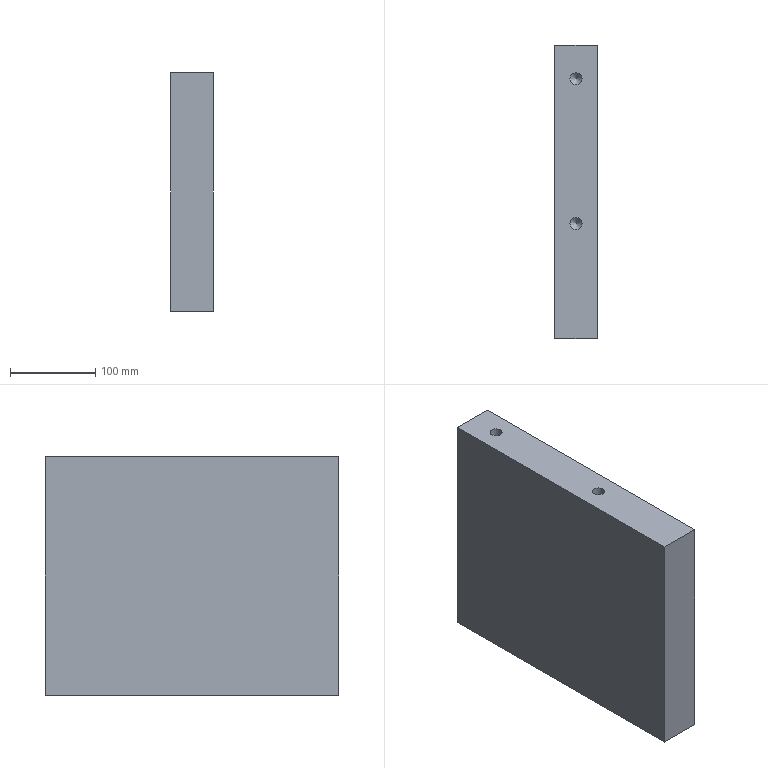Part | NX | features 29 2 | 1 solid | 14 faces | box 50 x 344.338 x 280.5 mm | volume 4804797 mm3 | plane 6 | cylinder 4 | cone 4 | commonest cylinder face diameters 14.1 x4
STEP:
#1=CARTESIAN_POINT('',(259.55,-367.5,-493.5));
#2=VERTEX_POINT('',#1);
#3=CARTESIAN_POINT('',(252.5,-367.5,-493.5));
#4=DIRECTION('',(0.,0.,1.));
#5=DIRECTION('',(1.,0.,0.));
#6=AXIS2_PLACEMENT_3D('',#3,#4,#5);
#7=CIRCLE('',#6,7.05);
#8=EDGE_CURVE('',#2,#2,#7,.T.);
#9=ORIENTED_EDGE('',*,*,#8,.T.);
#10=EDGE_LOOP('',(#9));
#11=FACE_BOUND('',#10,.T.);
#12=CARTESIAN_POINT('',(227.5,-328.162,-493.5));
#13=VERTEX_POINT('',#12);
#14=CARTESIAN_POINT('',(227.5,-672.5,-493.5));
#15=VERTEX_POINT('',#14);
#16=CARTESIAN_POINT('',(227.5,193.,-493.5));
#17=DIRECTION('',(0.,-1.,0.));
#18=VECTOR('',#17,1000.);
#19=LINE('',#16,#18);
#20=EDGE_CURVE('',#13,#15,#19,.T.);
#21=ORIENTED_EDGE('',*,*,#20,.F.);
#22=CARTESIAN_POINT('',(277.5,-328.162,-493.5));
#23=VERTEX_POINT('',#22);
#24=CARTESIAN_POINT('',(1945.,-328.162,-493.5));
#25=DIRECTION('',(1.,0.,0.));
#26=VECTOR('',#25,1000.);
#27=LINE('',#24,#26);
#28=EDGE_CURVE('',#13,#23,#27,.T.);
#29=ORIENTED_EDGE('',*,*,#28,.T.);
#30=CARTESIAN_POINT('',(277.5,-672.5,-493.5));
#31=VERTEX_POINT('',#30);
#32=CARTESIAN_POINT('',(277.5,193.,-493.5));
#33=DIRECTION('',(0.,1.,0.));
#34=VECTOR('',#33,1000.);
#35=LINE('',#32,#34);
#36=EDGE_CURVE('',#31,#23,#35,.T.);
#37=ORIENTED_EDGE('',*,*,#36,.F.);
#38=CARTESIAN_POINT('',(172.5,-672.5,-493.5));
#39=DIRECTION('',(-1.,0.,0.));
#40=VECTOR('',#39,1000.);
#41=LINE('',#38,#40);
#42=EDGE_CURVE('',#31,#15,#41,.T.);
#43=ORIENTED_EDGE('',*,*,#42,.T.);
#44=EDGE_LOOP('',(#21,#29,#37,#43));
#45=FACE_BOUND('',#44,.T.);
#46=CARTESIAN_POINT('',(259.55,-617.5,-493.5));
#47=VERTEX_POINT('',#46);
#48=CARTESIAN_POINT('',(252.5,-617.5,-493.5));
#49=DIRECTION('',(0.,0.,1.));
#50=DIRECTION('',(1.,0.,0.));
#51=AXIS2_PLACEMENT_3D('',#48,#49,#50);
#52=CIRCLE('',#51,7.05);
#53=EDGE_CURVE('',#47,#47,#52,.T.);
#54=ORIENTED_EDGE('',*,*,#53,.T.);
#55=EDGE_LOOP('',(#54));
#56=FACE_BOUND('',#55,.T.);
#57=CARTESIAN_POINT('',(1945.,0.,-493.5));
#58=DIRECTION('',(0.,0.,-1.));
#59=DIRECTION('',(1.,0.,0.));
#60=AXIS2_PLACEMENT_3D('',#57,#58,#59);
#61=PLANE('',#60);
#62=ADVANCED_FACE('',(#11,#45,#56),#61,.T.);
#63=CARTESIAN_POINT('',(259.55,-537.5,-213.));
#64=VERTEX_POINT('',#63);
#65=CARTESIAN_POINT('',(252.5,-537.5,-213.));
#66=DIRECTION('',(0.,0.,-1.));
#67=DIRECTION('',(1.,0.,0.));
#68=AXIS2_PLACEMENT_3D('',#65,#66,#67);
#69=CIRCLE('',#68,7.05);
#70=EDGE_CURVE('',#64,#64,#69,.T.);
#71=ORIENTED_EDGE('',*,*,#70,.T.);
#72=EDGE_LOOP('',(#71));
#73=FACE_BOUND('',#72,.T.);
#74=CARTESIAN_POINT('',(277.5,-328.162,-213.));
#75=VERTEX_POINT('',#74);
#76=CARTESIAN_POINT('',(277.5,-672.5,-213.));
#77=VERTEX_POINT('',#76);
#78=CARTESIAN_POINT('',(277.5,193.,-213.));
#79=DIRECTION('',(0.,-1.,0.));
#80=VECTOR('',#79,1000.);
#81=LINE('',#78,#80);
#82=EDGE_CURVE('',#75,#77,#81,.T.);
#83=ORIENTED_EDGE('',*,*,#82,.F.);
#84=CARTESIAN_POINT('',(227.5,-328.162,-213.));
#85=VERTEX_POINT('',#84);
#86=CARTESIAN_POINT('',(1945.,-328.162,-213.));
#87=DIRECTION('',(-1.,0.,0.));
#88=VECTOR('',#87,1000.);
#89=LINE('',#86,#88);
#90=EDGE_CURVE('',#75,#85,#89,.T.);
#91=ORIENTED_EDGE('',*,*,#90,.T.);
#92=CARTESIAN_POINT('',(227.5,-672.5,-213.));
#93=VERTEX_POINT('',#92);
#94=CARTESIAN_POINT('',(227.5,193.,-213.));
#95=DIRECTION('',(0.,1.,0.));
#96=VECTOR('',#95,1000.);
#97=LINE('',#94,#96);
#98=EDGE_CURVE('',#93,#85,#97,.T.);
#99=ORIENTED_EDGE('',*,*,#98,.F.);
#100=CARTESIAN_POINT('',(172.5,-672.5,-213.));
#101=DIRECTION('',(1.,0.,0.));
#102=VECTOR('',#101,1000.);
#103=LINE('',#100,#102);
#104=EDGE_CURVE('',#93,#77,#103,.T.);
#105=ORIENTED_EDGE('',*,*,#104,.T.);
#106=EDGE_LOOP('',(#83,#91,#99,#105));
#107=FACE_BOUND('',#106,.T.);
#108=CARTESIAN_POINT('',(259.55,-367.5,-213.));
#109=VERTEX_POINT('',#108);
#110=CARTESIAN_POINT('',(252.5,-367.5,-213.));
#111=DIRECTION('',(0.,0.,-1.));
#112=DIRECTION('',(1.,0.,0.));
#113=AXIS2_PLACEMENT_3D('',#110,#111,#112);
#114=CIRCLE('',#113,7.05);
#115=EDGE_CURVE('',#109,#109,#114,.T.);
#116=ORIENTED_EDGE('',*,*,#115,.T.);
#117=EDGE_LOOP('',(#116));
#118=FACE_BOUND('',#117,.T.);
#119=CARTESIAN_POINT('',(1945.,0.,-213.));
#120=DIRECTION('',(0.,0.,1.));
#121=DIRECTION('',(-1.,0.,0.));
#122=AXIS2_PLACEMENT_3D('',#119,#120,#121);
#123=PLANE('',#122);
#124=ADVANCED_FACE('',(#73,#107,#118),#123,.T.);
#125=ORIENTED_EDGE('',*,*,#28,.F.);
#126=CARTESIAN_POINT('',(227.5,-328.162,-205.5));
#127=DIRECTION('',(0.,0.,-1.));
#128=VECTOR('',#127,1000.);
#129=LINE('',#126,#128);
#130=EDGE_CURVE('',#85,#13,#129,.T.);
#131=ORIENTED_EDGE('',*,*,#130,.F.);
#132=ORIENTED_EDGE('',*,*,#90,.F.);
#133=CARTESIAN_POINT('',(277.5,-328.162,-205.5));
#134=DIRECTION('',(0.,0.,1.));
#135=VECTOR('',#134,1000.);
#136=LINE('',#133,#135);
#137=EDGE_CURVE('',#23,#75,#136,.T.);
#138=ORIENTED_EDGE('',*,*,#137,.F.);
#139=EDGE_LOOP('',(#125,#131,#132,#138));
#140=FACE_BOUND('',#139,.T.);
#141=CARTESIAN_POINT('',(343.,-328.162,-353.25));
#142=DIRECTION('',(0.,1.,0.));
#143=DIRECTION('',(0.,0.,-1.));
#144=AXIS2_PLACEMENT_3D('',#141,#142,#143);
#145=PLANE('',#144);
#146=ADVANCED_FACE('',(#140),#145,.T.);
#147=ORIENTED_EDGE('',*,*,#36,.T.);
#148=ORIENTED_EDGE('',*,*,#137,.T.);
#149=ORIENTED_EDGE('',*,*,#82,.T.);
#150=CARTESIAN_POINT('',(277.5,-672.5,-205.5));
#151=DIRECTION('',(0.,0.,1.));
#152=VECTOR('',#151,1000.);
#153=LINE('',#150,#152);
#154=EDGE_CURVE('',#31,#77,#153,.T.);
#155=ORIENTED_EDGE('',*,*,#154,.F.);
#156=EDGE_LOOP('',(#147,#148,#149,#155));
#157=FACE_BOUND('',#156,.T.);
#158=CARTESIAN_POINT('',(277.5,193.,-205.5));
#159=DIRECTION('',(1.,0.,0.));
#160=DIRECTION('',(0.,0.,-1.));
#161=AXIS2_PLACEMENT_3D('',#158,#159,#160);
#162=PLANE('',#161);
#163=ADVANCED_FACE('',(#157),#162,.T.);
#164=ORIENTED_EDGE('',*,*,#98,.T.);
#165=ORIENTED_EDGE('',*,*,#130,.T.);
#166=ORIENTED_EDGE('',*,*,#20,.T.);
#167=CARTESIAN_POINT('',(227.5,-672.5,-113.));
#168=DIRECTION('',(0.,0.,1.));
#169=VECTOR('',#168,1000.);
#170=LINE('',#167,#169);
#171=EDGE_CURVE('',#15,#93,#170,.T.);
#172=ORIENTED_EDGE('',*,*,#171,.T.);
#173=EDGE_LOOP('',(#164,#165,#166,#172));
#174=FACE_BOUND('',#173,.T.);
#175=CARTESIAN_POINT('',(227.5,193.,-205.5));
#176=DIRECTION('',(-1.,0.,0.));
#177=DIRECTION('',(0.,0.,1.));
#178=AXIS2_PLACEMENT_3D('',#175,#176,#177);
#179=PLANE('',#178);
#180=ADVANCED_FACE('',(#174),#179,.T.);
#181=ORIENTED_EDGE('',*,*,#42,.F.);
#182=ORIENTED_EDGE('',*,*,#154,.T.);
#183=ORIENTED_EDGE('',*,*,#104,.F.);
#184=ORIENTED_EDGE('',*,*,#171,.F.);
#185=EDGE_LOOP('',(#181,#182,#183,#184));
#186=FACE_BOUND('',#185,.T.);
#187=CARTESIAN_POINT('',(172.5,-672.5,-113.));
#188=DIRECTION('',(0.,1.,0.));
#189=DIRECTION('',(1.,0.,0.));
#190=AXIS2_PLACEMENT_3D('',#187,#188,#189);
#191=PLANE('',#190);
#192=ADVANCED_FACE('',(#186),#191,.F.);
#193=CARTESIAN_POINT('',(245.45,-537.5,-249.95));
#194=VERTEX_POINT('',#193);
#195=CARTESIAN_POINT('',(252.5,-537.5,-249.95));
#196=DIRECTION('',(0.,0.,-1.));
#197=DIRECTION('',(-1.,0.,0.));
#198=AXIS2_PLACEMENT_3D('',#195,#196,#197);
#199=CIRCLE('',#198,7.05);
#200=EDGE_CURVE('',#194,#194,#199,.T.);
#201=ORIENTED_EDGE('',*,*,#200,.T.);
#202=EDGE_LOOP('',(#201));
#203=FACE_BOUND('',#202,.T.);
#204=ORIENTED_EDGE('',*,*,#70,.F.);
#205=EDGE_LOOP('',(#204));
#206=FACE_BOUND('',#205,.T.);
#207=CARTESIAN_POINT('',(252.5,-537.5,-213.));
#208=DIRECTION('',(0.,0.,-1.));
#209=DIRECTION('',(-1.,0.,0.));
#210=AXIS2_PLACEMENT_3D('',#207,#208,#209);
#211=CYLINDRICAL_SURFACE('',#210,7.05);
#212=ADVANCED_FACE('',(#203,#206),#211,.F.);
#213=CARTESIAN_POINT('',(252.5,-537.5,-257.));
#214=VERTEX_POINT('',#213);
#215=VERTEX_LOOP('',#214);
#216=FACE_BOUND('',#215,.T.);
#217=ORIENTED_EDGE('',*,*,#200,.F.);
#218=EDGE_LOOP('',(#217));
#219=FACE_BOUND('',#218,.T.);
#220=CARTESIAN_POINT('',(252.5,-537.5,-249.95));
#221=DIRECTION('',(0.,0.,1.));
#222=DIRECTION('',(-1.,0.,0.));
#223=AXIS2_PLACEMENT_3D('',#220,#221,#222);
#224=CONICAL_SURFACE('',#223,7.05,0.7854);
#225=ADVANCED_FACE('',(#216,#219),#224,.F.);
#226=CARTESIAN_POINT('',(245.45,-367.5,-249.95));
#227=VERTEX_POINT('',#226);
#228=CARTESIAN_POINT('',(252.5,-367.5,-249.95));
#229=DIRECTION('',(0.,0.,-1.));
#230=DIRECTION('',(-1.,0.,0.));
#231=AXIS2_PLACEMENT_3D('',#228,#229,#230);
#232=CIRCLE('',#231,7.05);
#233=EDGE_CURVE('',#227,#227,#232,.T.);
#234=ORIENTED_EDGE('',*,*,#233,.T.);
#235=EDGE_LOOP('',(#234));
#236=FACE_BOUND('',#235,.T.);
#237=ORIENTED_EDGE('',*,*,#115,.F.);
#238=EDGE_LOOP('',(#237));
#239=FACE_BOUND('',#238,.T.);
#240=CARTESIAN_POINT('',(252.5,-367.5,-213.));
#241=DIRECTION('',(0.,0.,-1.));
#242=DIRECTION('',(-1.,0.,0.));
#243=AXIS2_PLACEMENT_3D('',#240,#241,#242);
#244=CYLINDRICAL_SURFACE('',#243,7.05);
#245=ADVANCED_FACE('',(#236,#239),#244,.F.);
#246=CARTESIAN_POINT('',(252.5,-367.5,-257.));
#247=VERTEX_POINT('',#246);
#248=VERTEX_LOOP('',#247);
#249=FACE_BOUND('',#248,.T.);
#250=ORIENTED_EDGE('',*,*,#233,.F.);
#251=EDGE_LOOP('',(#250));
#252=FACE_BOUND('',#251,.T.);
#253=CARTESIAN_POINT('',(252.5,-367.5,-249.95));
#254=DIRECTION('',(0.,0.,1.));
#255=DIRECTION('',(-1.,0.,0.));
#256=AXIS2_PLACEMENT_3D('',#253,#254,#255);
#257=CONICAL_SURFACE('',#256,7.05,0.7854);
#258=ADVANCED_FACE('',(#249,#252),#257,.F.);
#259=CARTESIAN_POINT('',(259.55,-367.5,-456.55));
#260=VERTEX_POINT('',#259);
#261=CARTESIAN_POINT('',(252.5,-367.5,-456.55));
#262=DIRECTION('',(0.,0.,1.));
#263=DIRECTION('',(1.,0.,0.));
#264=AXIS2_PLACEMENT_3D('',#261,#262,#263);
#265=CIRCLE('',#264,7.05);
#266=EDGE_CURVE('',#260,#260,#265,.T.);
#267=ORIENTED_EDGE('',*,*,#266,.T.);
#268=EDGE_LOOP('',(#267));
#269=FACE_BOUND('',#268,.T.);
#270=ORIENTED_EDGE('',*,*,#8,.F.);
#271=EDGE_LOOP('',(#270));
#272=FACE_BOUND('',#271,.T.);
#273=CARTESIAN_POINT('',(252.5,-367.5,-493.5));
#274=DIRECTION('',(0.,0.,1.));
#275=DIRECTION('',(-1.,0.,0.));
#276=AXIS2_PLACEMENT_3D('',#273,#274,#275);
#277=CYLINDRICAL_SURFACE('',#276,7.05);
#278=ADVANCED_FACE('',(#269,#272),#277,.F.);
#279=CARTESIAN_POINT('',(252.5,-367.5,-449.5));
#280=VERTEX_POINT('',#279);
#281=VERTEX_LOOP('',#280);
#282=FACE_BOUND('',#281,.T.);
#283=ORIENTED_EDGE('',*,*,#266,.F.);
#284=EDGE_LOOP('',(#283));
#285=FACE_BOUND('',#284,.T.);
#286=CARTESIAN_POINT('',(252.5,-367.5,-456.55));
#287=DIRECTION('',(0.,0.,-1.));
#288=DIRECTION('',(1.,0.,0.));
#289=AXIS2_PLACEMENT_3D('',#286,#287,#288);
#290=CONICAL_SURFACE('',#289,7.05,0.7854);
#291=ADVANCED_FACE('',(#282,#285),#290,.F.);
#292=CARTESIAN_POINT('',(259.55,-617.5,-456.55));
#293=VERTEX_POINT('',#292);
#294=CARTESIAN_POINT('',(252.5,-617.5,-456.55));
#295=DIRECTION('',(0.,0.,1.));
#296=DIRECTION('',(1.,0.,0.));
#297=AXIS2_PLACEMENT_3D('',#294,#295,#296);
#298=CIRCLE('',#297,7.05);
#299=EDGE_CURVE('',#293,#293,#298,.T.);
#300=ORIENTED_EDGE('',*,*,#299,.T.);
#301=EDGE_LOOP('',(#300));
#302=FACE_BOUND('',#301,.T.);
#303=ORIENTED_EDGE('',*,*,#53,.F.);
#304=EDGE_LOOP('',(#303));
#305=FACE_BOUND('',#304,.T.);
#306=CARTESIAN_POINT('',(252.5,-617.5,-493.5));
#307=DIRECTION('',(0.,0.,1.));
#308=DIRECTION('',(-1.,0.,0.));
#309=AXIS2_PLACEMENT_3D('',#306,#307,#308);
#310=CYLINDRICAL_SURFACE('',#309,7.05);
#311=ADVANCED_FACE('',(#302,#305),#310,.F.);
#312=CARTESIAN_POINT('',(252.5,-617.5,-449.5));
#313=VERTEX_POINT('',#312);
#314=VERTEX_LOOP('',#313);
#315=FACE_BOUND('',#314,.T.);
#316=ORIENTED_EDGE('',*,*,#299,.F.);
#317=EDGE_LOOP('',(#316));
#318=FACE_BOUND('',#317,.T.);
#319=CARTESIAN_POINT('',(252.5,-617.5,-456.55));
#320=DIRECTION('',(0.,0.,-1.));
#321=DIRECTION('',(1.,0.,0.));
#322=AXIS2_PLACEMENT_3D('',#319,#320,#321);
#323=CONICAL_SURFACE('',#322,7.05,0.7854);
#324=ADVANCED_FACE('',(#315,#318),#323,.F.);
#325=CLOSED_SHELL('',(#62,#124,#146,#163,#180,#192,#212,#225,#245,#258,#278,#291,#311,#324));
#326=MANIFOLD_SOLID_BREP('',#325);
#327=(LENGTH_UNIT()NAMED_UNIT(*)SI_UNIT(.MILLI.,.METRE.));
#328=UNCERTAINTY_MEASURE_WITH_UNIT(LENGTH_MEASURE(0.00001),#327,'','');
#329=(NAMED_UNIT(*)PLANE_ANGLE_UNIT()SI_UNIT($,.RADIAN.));
#330=(NAMED_UNIT(*)SI_UNIT($,.STERADIAN.)SOLID_ANGLE_UNIT());
#331=(GEOMETRIC_REPRESENTATION_CONTEXT(3)GLOBAL_UNCERTAINTY_ASSIGNED_CONTEXT((#328))GLOBAL_UNIT_ASSIGNED_CONTEXT((#327,#329,#330))REPRESENTATION_CONTEXT('',''));
#332=ADVANCED_BREP_SHAPE_REPRESENTATION('',(#326),#331);